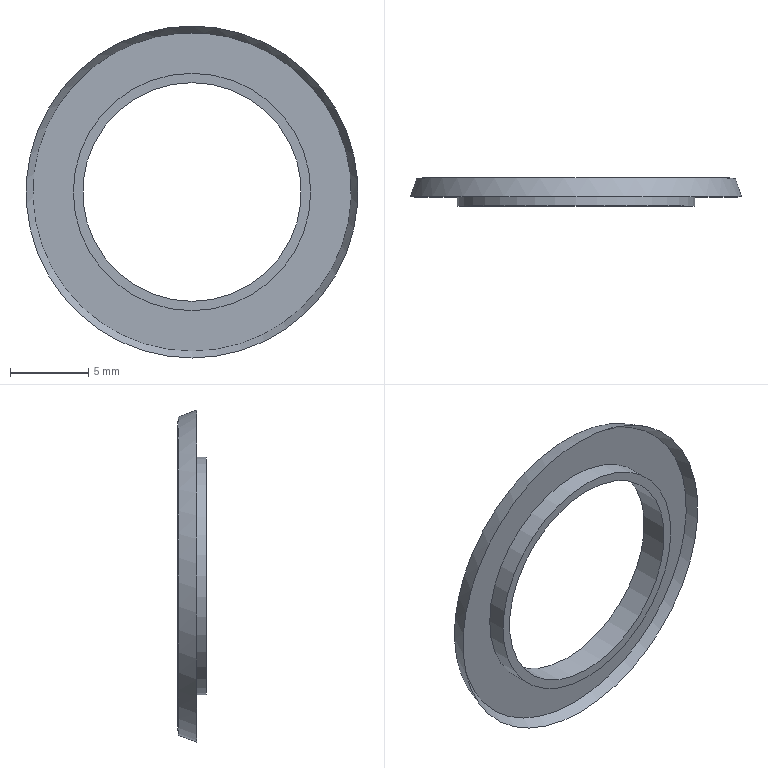Part | NX | features DATUM_CSYS 2, SKETCH 1, SWP104 1 | 1 solid | 8 faces | box 21.26 x 1.8 x 21.26 mm | volume 144.963 mm3 | plane 3 | cone 3 | cylinder 2 | commonest cylinder face diameters 14 x1 15.2 x1
STEP:
#1=CARTESIAN_POINT('',(0.,-0.6,-10.2));
#2=VERTEX_POINT('',#1);
#3=CARTESIAN_POINT('',(0.,-0.6,0.));
#4=DIRECTION('',(0.,-1.,0.));
#5=DIRECTION('',(0.,0.,-1.));
#6=AXIS2_PLACEMENT_3D('',#3,#4,#5);
#7=CIRCLE('',#6,10.2);
#8=EDGE_CURVE('',#2,#2,#7,.T.);
#9=ORIENTED_EDGE('',*,*,#8,.T.);
#10=EDGE_LOOP('',(#9));
#11=FACE_BOUND('',#10,.T.);
#12=CARTESIAN_POINT('',(0.,-0.6,-7.6));
#13=VERTEX_POINT('',#12);
#14=CARTESIAN_POINT('',(0.,-0.6,0.));
#15=DIRECTION('',(0.,-1.,0.));
#16=DIRECTION('',(0.,0.,-1.));
#17=AXIS2_PLACEMENT_3D('',#14,#15,#16);
#18=CIRCLE('',#17,7.6);
#19=EDGE_CURVE('',#13,#13,#18,.T.);
#20=ORIENTED_EDGE('',*,*,#19,.F.);
#21=EDGE_LOOP('',(#20));
#22=FACE_BOUND('',#21,.T.);
#23=CARTESIAN_POINT('',(0.,-0.6,7.6));
#24=DIRECTION('',(0.,-1.,0.));
#25=DIRECTION('',(0.,0.,-1.));
#26=AXIS2_PLACEMENT_3D('',#23,#24,#25);
#27=PLANE('',#26);
#28=ADVANCED_FACE('',(#11,#22),#27,.T.);
#29=CARTESIAN_POINT('',(0.,-1.214,-10.63));
#30=VERTEX_POINT('',#29);
#31=CARTESIAN_POINT('',(0.,-1.214,0.));
#32=DIRECTION('',(0.,-1.,0.));
#33=DIRECTION('',(0.,0.,-1.));
#34=AXIS2_PLACEMENT_3D('',#31,#32,#33);
#35=CIRCLE('',#34,10.63);
#36=EDGE_CURVE('',#30,#30,#35,.T.);
#37=ORIENTED_EDGE('',*,*,#36,.T.);
#38=EDGE_LOOP('',(#37));
#39=FACE_BOUND('',#38,.T.);
#40=ORIENTED_EDGE('',*,*,#8,.F.);
#41=EDGE_LOOP('',(#40));
#42=FACE_BOUND('',#41,.T.);
#43=CARTESIAN_POINT('',(0.,-0.6,0.));
#44=DIRECTION('',(0.,-1.,0.));
#45=DIRECTION('',(0.,0.,-1.));
#46=AXIS2_PLACEMENT_3D('',#43,#44,#45);
#47=CONICAL_SURFACE('',#46,10.2,0.6109);
#48=ADVANCED_FACE('',(#39,#42),#47,.F.);
#49=CARTESIAN_POINT('',(0.,-0.00711,-10.2));
#50=VERTEX_POINT('',#49);
#51=CARTESIAN_POINT('',(0.,-0.00711,0.));
#52=DIRECTION('',(0.,-1.,0.));
#53=DIRECTION('',(0.,0.,-1.));
#54=AXIS2_PLACEMENT_3D('',#51,#52,#53);
#55=CIRCLE('',#54,10.2);
#56=EDGE_CURVE('',#50,#50,#55,.T.);
#57=ORIENTED_EDGE('',*,*,#56,.T.);
#58=EDGE_LOOP('',(#57));
#59=FACE_BOUND('',#58,.T.);
#60=ORIENTED_EDGE('',*,*,#36,.F.);
#61=EDGE_LOOP('',(#60));
#62=FACE_BOUND('',#61,.T.);
#63=CARTESIAN_POINT('',(0.,-1.214,0.));
#64=DIRECTION('',(0.,-1.,0.));
#65=DIRECTION('',(0.,0.,-1.));
#66=AXIS2_PLACEMENT_3D('',#63,#64,#65);
#67=CONICAL_SURFACE('',#66,10.63,0.3423);
#68=ADVANCED_FACE('',(#59,#62),#67,.T.);
#69=CARTESIAN_POINT('',(0.,0.,-9.769));
#70=VERTEX_POINT('',#69);
#71=CARTESIAN_POINT('',(0.,0.,0.));
#72=DIRECTION('',(0.,-1.,0.));
#73=DIRECTION('',(0.,0.,-1.));
#74=AXIS2_PLACEMENT_3D('',#71,#72,#73);
#75=CIRCLE('',#74,9.769);
#76=EDGE_CURVE('',#70,#70,#75,.T.);
#77=ORIENTED_EDGE('',*,*,#76,.T.);
#78=EDGE_LOOP('',(#77));
#79=FACE_BOUND('',#78,.T.);
#80=ORIENTED_EDGE('',*,*,#56,.F.);
#81=EDGE_LOOP('',(#80));
#82=FACE_BOUND('',#81,.T.);
#83=CARTESIAN_POINT('',(0.,-0.00711,0.));
#84=DIRECTION('',(0.,-1.,0.));
#85=DIRECTION('',(0.,0.,-1.));
#86=AXIS2_PLACEMENT_3D('',#83,#84,#85);
#87=CONICAL_SURFACE('',#86,10.2,1.554);
#88=ADVANCED_FACE('',(#79,#82),#87,.T.);
#89=CARTESIAN_POINT('',(0.,0.,-7.));
#90=VERTEX_POINT('',#89);
#91=CARTESIAN_POINT('',(0.,0.,0.));
#92=DIRECTION('',(0.,-1.,0.));
#93=DIRECTION('',(0.,0.,-1.));
#94=AXIS2_PLACEMENT_3D('',#91,#92,#93);
#95=CIRCLE('',#94,7.);
#96=EDGE_CURVE('',#90,#90,#95,.T.);
#97=ORIENTED_EDGE('',*,*,#96,.T.);
#98=EDGE_LOOP('',(#97));
#99=FACE_BOUND('',#98,.T.);
#100=ORIENTED_EDGE('',*,*,#76,.F.);
#101=EDGE_LOOP('',(#100));
#102=FACE_BOUND('',#101,.T.);
#103=CARTESIAN_POINT('',(0.,0.,9.769));
#104=DIRECTION('',(0.,1.,0.));
#105=DIRECTION('',(0.,0.,1.));
#106=AXIS2_PLACEMENT_3D('',#103,#104,#105);
#107=PLANE('',#106);
#108=ADVANCED_FACE('',(#99,#102),#107,.T.);
#109=CARTESIAN_POINT('',(0.,-1.8,-7.));
#110=VERTEX_POINT('',#109);
#111=CARTESIAN_POINT('',(0.,-1.8,0.));
#112=DIRECTION('',(0.,-1.,0.));
#113=DIRECTION('',(0.,0.,-1.));
#114=AXIS2_PLACEMENT_3D('',#111,#112,#113);
#115=CIRCLE('',#114,7.);
#116=EDGE_CURVE('',#110,#110,#115,.T.);
#117=ORIENTED_EDGE('',*,*,#116,.T.);
#118=EDGE_LOOP('',(#117));
#119=FACE_BOUND('',#118,.T.);
#120=ORIENTED_EDGE('',*,*,#96,.F.);
#121=EDGE_LOOP('',(#120));
#122=FACE_BOUND('',#121,.T.);
#123=CARTESIAN_POINT('',(0.,0.,0.));
#124=DIRECTION('',(0.,-1.,0.));
#125=DIRECTION('',(0.,0.,-1.));
#126=AXIS2_PLACEMENT_3D('',#123,#124,#125);
#127=CYLINDRICAL_SURFACE('',#126,7.);
#128=ADVANCED_FACE('',(#119,#122),#127,.F.);
#129=CARTESIAN_POINT('',(0.,-1.8,-7.6));
#130=VERTEX_POINT('',#129);
#131=CARTESIAN_POINT('',(0.,-1.8,0.));
#132=DIRECTION('',(0.,-1.,0.));
#133=DIRECTION('',(0.,0.,-1.));
#134=AXIS2_PLACEMENT_3D('',#131,#132,#133);
#135=CIRCLE('',#134,7.6);
#136=EDGE_CURVE('',#130,#130,#135,.T.);
#137=ORIENTED_EDGE('',*,*,#136,.T.);
#138=EDGE_LOOP('',(#137));
#139=FACE_BOUND('',#138,.T.);
#140=ORIENTED_EDGE('',*,*,#116,.F.);
#141=EDGE_LOOP('',(#140));
#142=FACE_BOUND('',#141,.T.);
#143=CARTESIAN_POINT('',(0.,-1.8,7.));
#144=DIRECTION('',(0.,-1.,0.));
#145=DIRECTION('',(0.,0.,-1.));
#146=AXIS2_PLACEMENT_3D('',#143,#144,#145);
#147=PLANE('',#146);
#148=ADVANCED_FACE('',(#139,#142),#147,.T.);
#149=ORIENTED_EDGE('',*,*,#19,.T.);
#150=EDGE_LOOP('',(#149));
#151=FACE_BOUND('',#150,.T.);
#152=ORIENTED_EDGE('',*,*,#136,.F.);
#153=EDGE_LOOP('',(#152));
#154=FACE_BOUND('',#153,.T.);
#155=CARTESIAN_POINT('',(0.,0.,0.));
#156=DIRECTION('',(0.,-1.,0.));
#157=DIRECTION('',(0.,0.,-1.));
#158=AXIS2_PLACEMENT_3D('',#155,#156,#157);
#159=CYLINDRICAL_SURFACE('',#158,7.6);
#160=ADVANCED_FACE('',(#151,#154),#159,.T.);
#161=CLOSED_SHELL('',(#28,#48,#68,#88,#108,#128,#148,#160));
#162=MANIFOLD_SOLID_BREP('',#161);
#163=(LENGTH_UNIT()NAMED_UNIT(*)SI_UNIT(.MILLI.,.METRE.));
#164=UNCERTAINTY_MEASURE_WITH_UNIT(LENGTH_MEASURE(0.00001),#163,'','');
#165=(NAMED_UNIT(*)PLANE_ANGLE_UNIT()SI_UNIT($,.RADIAN.));
#166=(NAMED_UNIT(*)SI_UNIT($,.STERADIAN.)SOLID_ANGLE_UNIT());
#167=(GEOMETRIC_REPRESENTATION_CONTEXT(3)GLOBAL_UNCERTAINTY_ASSIGNED_CONTEXT((#164))GLOBAL_UNIT_ASSIGNED_CONTEXT((#163,#165,#166))REPRESENTATION_CONTEXT('',''));
#168=ADVANCED_BREP_SHAPE_REPRESENTATION('',(#162),#167);